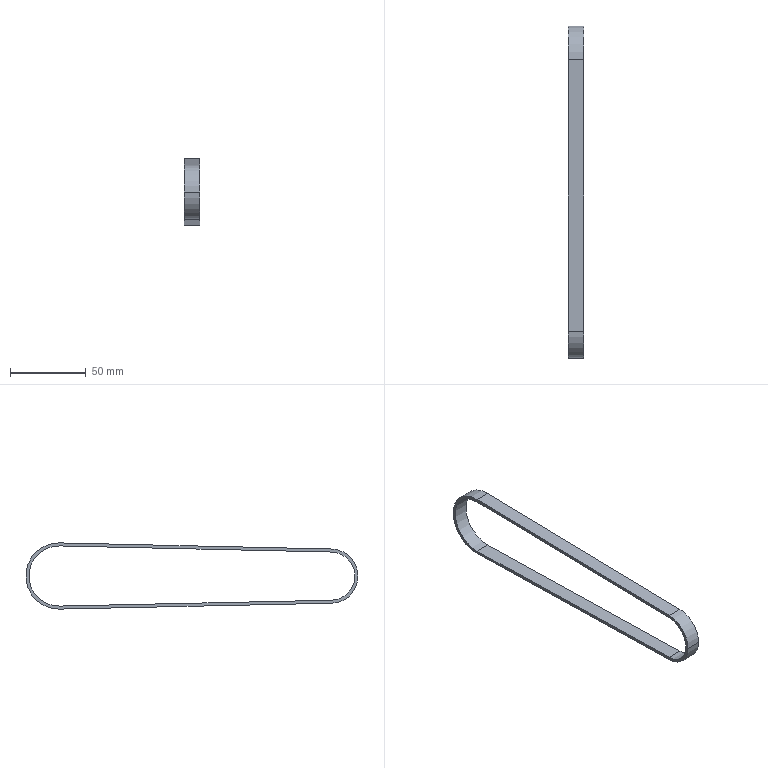Part | NX | 1 solid | 12 faces | box 10 x 219.471 x 43.75 mm | volume 9563 mm3 | plane 6 | cylinder 6 | commonest cylinder face diameters 31.83 x2 35.83 x2 39.75 x1 43.75 x1
STEP:
#1=CARTESIAN_POINT('',(2252.5,160.553,-22.13));
#2=VERTEX_POINT('',#1);
#3=CARTESIAN_POINT('',(2252.5,-19.038,-26.166));
#4=VERTEX_POINT('',#3);
#5=CARTESIAN_POINT('',(2252.5,160.553,-22.13));
#6=DIRECTION('',(0.,-0.9997,-0.02247));
#7=VECTOR('',#6,1000.);
#8=LINE('',#5,#7);
#9=EDGE_CURVE('',#2,#4,#8,.T.);
#10=ORIENTED_EDGE('',*,*,#9,.F.);
#11=CARTESIAN_POINT('',(2262.5,160.553,-22.13));
#12=VERTEX_POINT('',#11);
#13=CARTESIAN_POINT('',(2252.5,160.553,-22.13));
#14=DIRECTION('',(1.,0.,0.));
#15=VECTOR('',#14,1000.);
#16=LINE('',#13,#15);
#17=EDGE_CURVE('',#2,#12,#16,.T.);
#18=ORIENTED_EDGE('',*,*,#17,.T.);
#19=CARTESIAN_POINT('',(2262.5,-19.038,-26.166));
#20=VERTEX_POINT('',#19);
#21=CARTESIAN_POINT('',(2262.5,160.553,-22.13));
#22=DIRECTION('',(0.,-0.9997,-0.02247));
#23=VECTOR('',#22,1000.);
#24=LINE('',#21,#23);
#25=EDGE_CURVE('',#12,#20,#24,.T.);
#26=ORIENTED_EDGE('',*,*,#25,.T.);
#27=CARTESIAN_POINT('',(2252.5,-19.038,-26.166));
#28=DIRECTION('',(1.,0.,0.));
#29=VECTOR('',#28,1000.);
#30=LINE('',#27,#29);
#31=EDGE_CURVE('',#4,#20,#30,.T.);
#32=ORIENTED_EDGE('',*,*,#31,.F.);
#33=EDGE_LOOP('',(#10,#18,#26,#32));
#34=FACE_BOUND('',#33,.T.);
#35=CARTESIAN_POINT('',(2252.5,160.553,-22.13));
#36=DIRECTION('',(0.,0.02247,-0.9997));
#37=DIRECTION('',(-1.,0.,0.));
#38=AXIS2_PLACEMENT_3D('',#35,#36,#37);
#39=PLANE('',#38);
#40=ADVANCED_FACE('',(#34),#39,.T.);
#41=CARTESIAN_POINT('',(2252.5,160.571,-61.87));
#42=VERTEX_POINT('',#41);
#43=CARTESIAN_POINT('',(2252.5,161.,-42.));
#44=DIRECTION('',(-1.,0.,0.));
#45=DIRECTION('',(0.,-1.,0.));
#46=AXIS2_PLACEMENT_3D('',#43,#44,#45);
#47=CIRCLE('',#46,19.875);
#48=EDGE_CURVE('',#2,#42,#47,.T.);
#49=ORIENTED_EDGE('',*,*,#48,.T.);
#50=CARTESIAN_POINT('',(2262.5,160.571,-61.87));
#51=VERTEX_POINT('',#50);
#52=CARTESIAN_POINT('',(2252.5,160.571,-61.87));
#53=DIRECTION('',(1.,0.,0.));
#54=VECTOR('',#53,1000.);
#55=LINE('',#52,#54);
#56=EDGE_CURVE('',#42,#51,#55,.T.);
#57=ORIENTED_EDGE('',*,*,#56,.T.);
#58=CARTESIAN_POINT('',(2262.5,161.,-42.));
#59=DIRECTION('',(-1.,0.,0.));
#60=DIRECTION('',(0.,-1.,0.));
#61=AXIS2_PLACEMENT_3D('',#58,#59,#60);
#62=CIRCLE('',#61,19.875);
#63=EDGE_CURVE('',#12,#51,#62,.T.);
#64=ORIENTED_EDGE('',*,*,#63,.F.);
#65=ORIENTED_EDGE('',*,*,#17,.F.);
#66=EDGE_LOOP('',(#49,#57,#64,#65));
#67=FACE_BOUND('',#66,.T.);
#68=CARTESIAN_POINT('',(2252.5,161.,-42.));
#69=DIRECTION('',(-1.,0.,0.));
#70=DIRECTION('',(0.,-1.,0.));
#71=AXIS2_PLACEMENT_3D('',#68,#69,#70);
#72=CYLINDRICAL_SURFACE('',#71,19.875);
#73=ADVANCED_FACE('',(#67),#72,.F.);
#74=CARTESIAN_POINT('',(2252.5,-19.025,-57.989));
#75=VERTEX_POINT('',#74);
#76=CARTESIAN_POINT('',(2252.5,160.571,-61.87));
#77=DIRECTION('',(0.,-0.9998,0.02161));
#78=VECTOR('',#77,1000.);
#79=LINE('',#76,#78);
#80=EDGE_CURVE('',#42,#75,#79,.T.);
#81=ORIENTED_EDGE('',*,*,#80,.T.);
#82=CARTESIAN_POINT('',(2262.5,-19.025,-57.989));
#83=VERTEX_POINT('',#82);
#84=CARTESIAN_POINT('',(2252.5,-19.025,-57.989));
#85=DIRECTION('',(1.,0.,0.));
#86=VECTOR('',#85,1000.);
#87=LINE('',#84,#86);
#88=EDGE_CURVE('',#75,#83,#87,.T.);
#89=ORIENTED_EDGE('',*,*,#88,.T.);
#90=CARTESIAN_POINT('',(2262.5,160.571,-61.87));
#91=DIRECTION('',(0.,-0.9998,0.02161));
#92=VECTOR('',#91,1000.);
#93=LINE('',#90,#92);
#94=EDGE_CURVE('',#51,#83,#93,.T.);
#95=ORIENTED_EDGE('',*,*,#94,.F.);
#96=ORIENTED_EDGE('',*,*,#56,.F.);
#97=EDGE_LOOP('',(#81,#89,#95,#96));
#98=FACE_BOUND('',#97,.T.);
#99=CARTESIAN_POINT('',(2252.5,-19.025,-57.989));
#100=DIRECTION('',(0.,0.02161,0.9998));
#101=DIRECTION('',(1.,0.,0.));
#102=AXIS2_PLACEMENT_3D('',#99,#100,#101);
#103=PLANE('',#102);
#104=ADVANCED_FACE('',(#98),#103,.T.);
#105=CARTESIAN_POINT('',(2262.5,-34.596,-42.077));
#106=VERTEX_POINT('',#105);
#107=CARTESIAN_POINT('',(2252.5,-34.596,-42.077));
#108=VERTEX_POINT('',#107);
#109=CARTESIAN_POINT('',(2252.5,-34.596,-42.077));
#110=DIRECTION('',(-1.,0.,0.));
#111=VECTOR('',#110,1000.);
#112=LINE('',#109,#111);
#113=EDGE_CURVE('',#106,#108,#112,.T.);
#114=ORIENTED_EDGE('',*,*,#113,.F.);
#115=CARTESIAN_POINT('',(2262.5,-18.681,-42.077));
#116=DIRECTION('',(-1.,0.,0.));
#117=DIRECTION('',(0.,-1.,0.));
#118=AXIS2_PLACEMENT_3D('',#115,#116,#117);
#119=CIRCLE('',#118,15.915);
#120=EDGE_CURVE('',#83,#106,#119,.T.);
#121=ORIENTED_EDGE('',*,*,#120,.F.);
#122=ORIENTED_EDGE('',*,*,#88,.F.);
#123=CARTESIAN_POINT('',(2252.5,-18.681,-42.077));
#124=DIRECTION('',(-1.,0.,0.));
#125=DIRECTION('',(0.,-1.,0.));
#126=AXIS2_PLACEMENT_3D('',#123,#124,#125);
#127=CIRCLE('',#126,15.915);
#128=EDGE_CURVE('',#75,#108,#127,.T.);
#129=ORIENTED_EDGE('',*,*,#128,.T.);
#130=EDGE_LOOP('',(#114,#121,#122,#129));
#131=FACE_BOUND('',#130,.T.);
#132=CARTESIAN_POINT('',(2252.5,-18.681,-42.077));
#133=DIRECTION('',(-1.,0.,0.));
#134=DIRECTION('',(0.,-1.,0.));
#135=AXIS2_PLACEMENT_3D('',#132,#133,#134);
#136=CYLINDRICAL_SURFACE('',#135,15.915);
#137=ADVANCED_FACE('',(#131),#136,.F.);
#138=CARTESIAN_POINT('',(2252.5,160.508,-20.131));
#139=VERTEX_POINT('',#138);
#140=CARTESIAN_POINT('',(2252.5,-19.083,-24.167));
#141=VERTEX_POINT('',#140);
#142=CARTESIAN_POINT('',(2252.5,160.508,-20.131));
#143=DIRECTION('',(0.,-0.9997,-0.02247));
#144=VECTOR('',#143,1000.);
#145=LINE('',#142,#144);
#146=EDGE_CURVE('',#139,#141,#145,.T.);
#147=ORIENTED_EDGE('',*,*,#146,.T.);
#148=CARTESIAN_POINT('',(2262.5,-19.083,-24.167));
#149=VERTEX_POINT('',#148);
#150=CARTESIAN_POINT('',(2252.5,-19.083,-24.167));
#151=DIRECTION('',(1.,0.,0.));
#152=VECTOR('',#151,1000.);
#153=LINE('',#150,#152);
#154=EDGE_CURVE('',#141,#149,#153,.T.);
#155=ORIENTED_EDGE('',*,*,#154,.T.);
#156=CARTESIAN_POINT('',(2262.5,160.508,-20.131));
#157=VERTEX_POINT('',#156);
#158=CARTESIAN_POINT('',(2262.5,160.508,-20.131));
#159=DIRECTION('',(0.,-0.9997,-0.02247));
#160=VECTOR('',#159,1000.);
#161=LINE('',#158,#160);
#162=EDGE_CURVE('',#157,#149,#161,.T.);
#163=ORIENTED_EDGE('',*,*,#162,.F.);
#164=CARTESIAN_POINT('',(2252.5,160.508,-20.131));
#165=DIRECTION('',(1.,0.,0.));
#166=VECTOR('',#165,1000.);
#167=LINE('',#164,#166);
#168=EDGE_CURVE('',#139,#157,#167,.T.);
#169=ORIENTED_EDGE('',*,*,#168,.F.);
#170=EDGE_LOOP('',(#147,#155,#163,#169));
#171=FACE_BOUND('',#170,.T.);
#172=CARTESIAN_POINT('',(2252.5,-19.083,-24.167));
#173=DIRECTION('',(0.,-0.02247,0.9997));
#174=DIRECTION('',(-1.,0.,0.));
#175=AXIS2_PLACEMENT_3D('',#172,#173,#174);
#176=PLANE('',#175);
#177=ADVANCED_FACE('',(#171),#176,.T.);
#178=CARTESIAN_POINT('',(2262.5,-36.596,-42.077));
#179=VERTEX_POINT('',#178);
#180=CARTESIAN_POINT('',(2252.5,-36.596,-42.077));
#181=VERTEX_POINT('',#180);
#182=CARTESIAN_POINT('',(2252.5,-36.596,-42.077));
#183=DIRECTION('',(-1.,0.,0.));
#184=VECTOR('',#183,1000.);
#185=LINE('',#182,#184);
#186=EDGE_CURVE('',#179,#181,#185,.T.);
#187=ORIENTED_EDGE('',*,*,#186,.F.);
#188=CARTESIAN_POINT('',(2262.5,-18.681,-42.077));
#189=DIRECTION('',(-1.,0.,0.));
#190=DIRECTION('',(0.,-1.,0.));
#191=AXIS2_PLACEMENT_3D('',#188,#189,#190);
#192=CIRCLE('',#191,17.915);
#193=EDGE_CURVE('',#179,#149,#192,.T.);
#194=ORIENTED_EDGE('',*,*,#193,.T.);
#195=ORIENTED_EDGE('',*,*,#154,.F.);
#196=CARTESIAN_POINT('',(2252.5,-18.681,-42.077));
#197=DIRECTION('',(-1.,0.,0.));
#198=DIRECTION('',(0.,-1.,0.));
#199=AXIS2_PLACEMENT_3D('',#196,#197,#198);
#200=CIRCLE('',#199,17.915);
#201=EDGE_CURVE('',#181,#141,#200,.T.);
#202=ORIENTED_EDGE('',*,*,#201,.F.);
#203=EDGE_LOOP('',(#187,#194,#195,#202));
#204=FACE_BOUND('',#203,.T.);
#205=CARTESIAN_POINT('',(2252.5,-18.681,-42.077));
#206=DIRECTION('',(-1.,0.,0.));
#207=DIRECTION('',(0.,-1.,0.));
#208=AXIS2_PLACEMENT_3D('',#205,#206,#207);
#209=CYLINDRICAL_SURFACE('',#208,17.915);
#210=ADVANCED_FACE('',(#204),#209,.T.);
#211=CARTESIAN_POINT('',(2252.5,160.527,-63.87));
#212=VERTEX_POINT('',#211);
#213=CARTESIAN_POINT('',(2252.5,-19.068,-59.988));
#214=VERTEX_POINT('',#213);
#215=CARTESIAN_POINT('',(2252.5,160.527,-63.87));
#216=DIRECTION('',(0.,-0.9998,0.02161));
#217=VECTOR('',#216,1000.);
#218=LINE('',#215,#217);
#219=EDGE_CURVE('',#212,#214,#218,.T.);
#220=ORIENTED_EDGE('',*,*,#219,.F.);
#221=CARTESIAN_POINT('',(2262.5,160.527,-63.87));
#222=VERTEX_POINT('',#221);
#223=CARTESIAN_POINT('',(2252.5,160.527,-63.87));
#224=DIRECTION('',(1.,0.,0.));
#225=VECTOR('',#224,1000.);
#226=LINE('',#223,#225);
#227=EDGE_CURVE('',#212,#222,#226,.T.);
#228=ORIENTED_EDGE('',*,*,#227,.T.);
#229=CARTESIAN_POINT('',(2262.5,-19.068,-59.988));
#230=VERTEX_POINT('',#229);
#231=CARTESIAN_POINT('',(2262.5,160.527,-63.87));
#232=DIRECTION('',(0.,-0.9998,0.02161));
#233=VECTOR('',#232,1000.);
#234=LINE('',#231,#233);
#235=EDGE_CURVE('',#222,#230,#234,.T.);
#236=ORIENTED_EDGE('',*,*,#235,.T.);
#237=CARTESIAN_POINT('',(2252.5,-19.068,-59.988));
#238=DIRECTION('',(1.,0.,0.));
#239=VECTOR('',#238,1000.);
#240=LINE('',#237,#239);
#241=EDGE_CURVE('',#214,#230,#240,.T.);
#242=ORIENTED_EDGE('',*,*,#241,.F.);
#243=EDGE_LOOP('',(#220,#228,#236,#242));
#244=FACE_BOUND('',#243,.T.);
#245=CARTESIAN_POINT('',(2252.5,160.527,-63.87));
#246=DIRECTION('',(0.,-0.02161,-0.9998));
#247=DIRECTION('',(0.,-0.9998,0.02161));
#248=AXIS2_PLACEMENT_3D('',#245,#246,#247);
#249=PLANE('',#248);
#250=ADVANCED_FACE('',(#244),#249,.T.);
#251=CARTESIAN_POINT('',(2252.5,161.,-42.));
#252=DIRECTION('',(-1.,0.,0.));
#253=DIRECTION('',(0.,-1.,0.));
#254=AXIS2_PLACEMENT_3D('',#251,#252,#253);
#255=CIRCLE('',#254,21.875);
#256=EDGE_CURVE('',#139,#212,#255,.T.);
#257=ORIENTED_EDGE('',*,*,#256,.F.);
#258=ORIENTED_EDGE('',*,*,#168,.T.);
#259=CARTESIAN_POINT('',(2262.5,161.,-42.));
#260=DIRECTION('',(-1.,0.,0.));
#261=DIRECTION('',(0.,-1.,0.));
#262=AXIS2_PLACEMENT_3D('',#259,#260,#261);
#263=CIRCLE('',#262,21.875);
#264=EDGE_CURVE('',#157,#222,#263,.T.);
#265=ORIENTED_EDGE('',*,*,#264,.T.);
#266=ORIENTED_EDGE('',*,*,#227,.F.);
#267=EDGE_LOOP('',(#257,#258,#265,#266));
#268=FACE_BOUND('',#267,.T.);
#269=CARTESIAN_POINT('',(2252.5,161.,-42.));
#270=DIRECTION('',(-1.,0.,0.));
#271=DIRECTION('',(0.,-1.,0.));
#272=AXIS2_PLACEMENT_3D('',#269,#270,#271);
#273=CYLINDRICAL_SURFACE('',#272,21.875);
#274=ADVANCED_FACE('',(#268),#273,.T.);
#275=ORIENTED_EDGE('',*,*,#264,.F.);
#276=ORIENTED_EDGE('',*,*,#162,.T.);
#277=ORIENTED_EDGE('',*,*,#193,.F.);
#278=CARTESIAN_POINT('',(2262.5,-18.681,-42.077));
#279=DIRECTION('',(-1.,0.,0.));
#280=DIRECTION('',(0.,-1.,0.));
#281=AXIS2_PLACEMENT_3D('',#278,#279,#280);
#282=CIRCLE('',#281,17.915);
#283=EDGE_CURVE('',#230,#179,#282,.T.);
#284=ORIENTED_EDGE('',*,*,#283,.F.);
#285=ORIENTED_EDGE('',*,*,#235,.F.);
#286=EDGE_LOOP('',(#275,#276,#277,#284,#285));
#287=FACE_BOUND('',#286,.T.);
#288=ORIENTED_EDGE('',*,*,#94,.T.);
#289=ORIENTED_EDGE('',*,*,#120,.T.);
#290=CARTESIAN_POINT('',(2262.5,-18.681,-42.077));
#291=DIRECTION('',(-1.,0.,0.));
#292=DIRECTION('',(0.,-1.,0.));
#293=AXIS2_PLACEMENT_3D('',#290,#291,#292);
#294=CIRCLE('',#293,15.915);
#295=EDGE_CURVE('',#106,#20,#294,.T.);
#296=ORIENTED_EDGE('',*,*,#295,.T.);
#297=ORIENTED_EDGE('',*,*,#25,.F.);
#298=ORIENTED_EDGE('',*,*,#63,.T.);
#299=EDGE_LOOP('',(#288,#289,#296,#297,#298));
#300=FACE_BOUND('',#299,.T.);
#301=CARTESIAN_POINT('',(2262.5,96.972,-18.975));
#302=DIRECTION('',(-1.,0.,0.));
#303=DIRECTION('',(0.,0.,1.));
#304=AXIS2_PLACEMENT_3D('',#301,#302,#303);
#305=PLANE('',#304);
#306=ADVANCED_FACE('',(#287,#300),#305,.F.);
#307=ORIENTED_EDGE('',*,*,#219,.T.);
#308=CARTESIAN_POINT('',(2252.5,-18.681,-42.077));
#309=DIRECTION('',(-1.,0.,0.));
#310=DIRECTION('',(0.,-1.,0.));
#311=AXIS2_PLACEMENT_3D('',#308,#309,#310);
#312=CIRCLE('',#311,17.915);
#313=EDGE_CURVE('',#214,#181,#312,.T.);
#314=ORIENTED_EDGE('',*,*,#313,.T.);
#315=ORIENTED_EDGE('',*,*,#201,.T.);
#316=ORIENTED_EDGE('',*,*,#146,.F.);
#317=ORIENTED_EDGE('',*,*,#256,.T.);
#318=EDGE_LOOP('',(#307,#314,#315,#316,#317));
#319=FACE_BOUND('',#318,.T.);
#320=ORIENTED_EDGE('',*,*,#48,.F.);
#321=ORIENTED_EDGE('',*,*,#9,.T.);
#322=CARTESIAN_POINT('',(2252.5,-18.681,-42.077));
#323=DIRECTION('',(-1.,0.,0.));
#324=DIRECTION('',(0.,-1.,0.));
#325=AXIS2_PLACEMENT_3D('',#322,#323,#324);
#326=CIRCLE('',#325,15.915);
#327=EDGE_CURVE('',#108,#4,#326,.T.);
#328=ORIENTED_EDGE('',*,*,#327,.F.);
#329=ORIENTED_EDGE('',*,*,#128,.F.);
#330=ORIENTED_EDGE('',*,*,#80,.F.);
#331=EDGE_LOOP('',(#320,#321,#328,#329,#330));
#332=FACE_BOUND('',#331,.T.);
#333=CARTESIAN_POINT('',(2252.5,96.972,-18.975));
#334=DIRECTION('',(-1.,0.,0.));
#335=DIRECTION('',(0.,0.,1.));
#336=AXIS2_PLACEMENT_3D('',#333,#334,#335);
#337=PLANE('',#336);
#338=ADVANCED_FACE('',(#319,#332),#337,.T.);
#339=ORIENTED_EDGE('',*,*,#283,.T.);
#340=ORIENTED_EDGE('',*,*,#186,.T.);
#341=ORIENTED_EDGE('',*,*,#313,.F.);
#342=ORIENTED_EDGE('',*,*,#241,.T.);
#343=EDGE_LOOP('',(#339,#340,#341,#342));
#344=FACE_BOUND('',#343,.T.);
#345=CARTESIAN_POINT('',(2252.5,-18.681,-42.077));
#346=DIRECTION('',(-1.,0.,0.));
#347=DIRECTION('',(0.,-1.,0.));
#348=AXIS2_PLACEMENT_3D('',#345,#346,#347);
#349=CYLINDRICAL_SURFACE('',#348,17.915);
#350=ADVANCED_FACE('',(#344),#349,.T.);
#351=ORIENTED_EDGE('',*,*,#295,.F.);
#352=ORIENTED_EDGE('',*,*,#113,.T.);
#353=ORIENTED_EDGE('',*,*,#327,.T.);
#354=ORIENTED_EDGE('',*,*,#31,.T.);
#355=EDGE_LOOP('',(#351,#352,#353,#354));
#356=FACE_BOUND('',#355,.T.);
#357=CARTESIAN_POINT('',(2252.5,-18.681,-42.077));
#358=DIRECTION('',(-1.,0.,0.));
#359=DIRECTION('',(0.,-1.,0.));
#360=AXIS2_PLACEMENT_3D('',#357,#358,#359);
#361=CYLINDRICAL_SURFACE('',#360,15.915);
#362=ADVANCED_FACE('',(#356),#361,.F.);
#363=CLOSED_SHELL('',(#40,#73,#104,#137,#177,#210,#250,#274,#306,#338,#350,#362));
#364=MANIFOLD_SOLID_BREP('',#363);
#365=(LENGTH_UNIT()NAMED_UNIT(*)SI_UNIT(.MILLI.,.METRE.));
#366=UNCERTAINTY_MEASURE_WITH_UNIT(LENGTH_MEASURE(0.00001),#365,'','');
#367=(NAMED_UNIT(*)PLANE_ANGLE_UNIT()SI_UNIT($,.RADIAN.));
#368=(NAMED_UNIT(*)SI_UNIT($,.STERADIAN.)SOLID_ANGLE_UNIT());
#369=(GEOMETRIC_REPRESENTATION_CONTEXT(3)GLOBAL_UNCERTAINTY_ASSIGNED_CONTEXT((#366))GLOBAL_UNIT_ASSIGNED_CONTEXT((#365,#367,#368))REPRESENTATION_CONTEXT('',''));
#370=ADVANCED_BREP_SHAPE_REPRESENTATION('',(#364),#369);